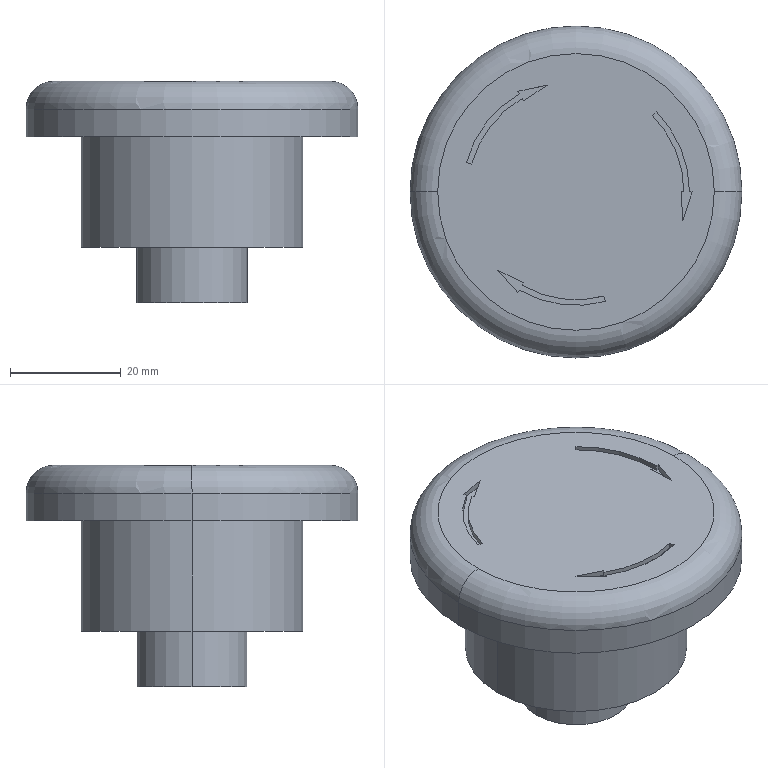Part | SolidWorks | features ICE 3, CirPattern 1, Extrusion 1, Fillet 1, Scale 1 | 1 solid | 36 faces | box 60 x 60 x 40 mm | volume 55512 mm3 | plane 22 | cylinder 12 | torus 2 | commonest cylinder face diameters 39 x3 41 x3 20 x2 40 x2 60 x2
STEP:
#1=CARTESIAN_POINT('',(-3.,0.,27.294));
#2=VERTEX_POINT('',#1);
#3=CARTESIAN_POINT('',(3.,0.,27.294));
#4=VERTEX_POINT('',#3);
#5=CARTESIAN_POINT('',(0.,0.,27.294));
#6=DIRECTION('',(0.,0.,-1.));
#7=DIRECTION('',(1.,0.,0.));
#8=AXIS2_PLACEMENT_3D('',#5,#6,#7);
#9=CIRCLE('',#8,3.);
#10=EDGE_CURVE('',#2,#4,#9,.T.);
#11=ORIENTED_EDGE('',*,*,#10,.F.);
#12=CARTESIAN_POINT('',(-2.5,0.,27.794));
#13=VERTEX_POINT('',#12);
#14=CARTESIAN_POINT('',(-2.5,0.,27.294));
#15=DIRECTION('',(0.,1.,0.));
#16=DIRECTION('',(-1.,0.,0.));
#17=AXIS2_PLACEMENT_3D('',#14,#15,#16);
#18=CIRCLE('',#17,0.5);
#19=EDGE_CURVE('',#2,#13,#18,.T.);
#20=ORIENTED_EDGE('',*,*,#19,.T.);
#21=CARTESIAN_POINT('',(2.5,0.,27.794));
#22=VERTEX_POINT('',#21);
#23=CARTESIAN_POINT('',(0.,0.,27.794));
#24=DIRECTION('',(0.,0.,1.));
#25=DIRECTION('',(1.,0.,0.));
#26=AXIS2_PLACEMENT_3D('',#23,#24,#25);
#27=CIRCLE('',#26,2.5);
#28=EDGE_CURVE('',#22,#13,#27,.T.);
#29=ORIENTED_EDGE('',*,*,#28,.F.);
#30=CARTESIAN_POINT('',(2.5,0.,27.294));
#31=DIRECTION('',(0.,-1.,0.));
#32=DIRECTION('',(0.,0.,-1.));
#33=AXIS2_PLACEMENT_3D('',#30,#31,#32);
#34=CIRCLE('',#33,0.5);
#35=EDGE_CURVE('',#4,#22,#34,.T.);
#36=ORIENTED_EDGE('',*,*,#35,.F.);
#37=EDGE_LOOP('',(#11,#20,#29,#36));
#38=FACE_OUTER_BOUND('',#37,.T.);
#39=CARTESIAN_POINT('',(0.,0.,27.294));
#40=DIRECTION('',(0.,0.,1.));
#41=DIRECTION('',(1.,0.,0.));
#42=AXIS2_PLACEMENT_3D('',#39,#40,#41);
#43=TOROIDAL_SURFACE('',#42,2.5,0.5);
#44=ADVANCED_FACE('',(#38),#43,.T.);
#45=ORIENTED_EDGE('',*,*,#10,.T.);
#46=CARTESIAN_POINT('',(3.,0.,26.794));
#47=VERTEX_POINT('',#46);
#48=CARTESIAN_POINT('',(3.,0.,27.794));
#49=DIRECTION('',(0.,0.,-1.));
#50=VECTOR('',#49,100.);
#51=LINE('',#48,#50);
#52=EDGE_CURVE('',#4,#47,#51,.T.);
#53=ORIENTED_EDGE('',*,*,#52,.T.);
#54=CARTESIAN_POINT('',(-3.,0.,26.794));
#55=VERTEX_POINT('',#54);
#56=CARTESIAN_POINT('',(0.,0.,26.794));
#57=DIRECTION('',(0.,0.,1.));
#58=DIRECTION('',(1.,0.,0.));
#59=AXIS2_PLACEMENT_3D('',#56,#57,#58);
#60=CIRCLE('',#59,3.);
#61=EDGE_CURVE('',#47,#55,#60,.T.);
#62=ORIENTED_EDGE('',*,*,#61,.T.);
#63=CARTESIAN_POINT('',(-3.,0.,27.794));
#64=DIRECTION('',(0.,0.,-1.));
#65=VECTOR('',#64,100.);
#66=LINE('',#63,#65);
#67=EDGE_CURVE('',#2,#55,#66,.T.);
#68=ORIENTED_EDGE('',*,*,#67,.F.);
#69=EDGE_LOOP('',(#45,#53,#62,#68));
#70=FACE_OUTER_BOUND('',#69,.T.);
#71=CARTESIAN_POINT('',(0.,0.,27.794));
#72=DIRECTION('',(0.,0.,-1.));
#73=DIRECTION('',(-1.,0.,0.));
#74=AXIS2_PLACEMENT_3D('',#71,#72,#73);
#75=CYLINDRICAL_SURFACE('',#74,3.);
#76=ADVANCED_FACE('',(#70),#75,.T.);
#77=CARTESIAN_POINT('',(2.,0.,26.794));
#78=VERTEX_POINT('',#77);
#79=CARTESIAN_POINT('',(-2.,0.,26.794));
#80=VERTEX_POINT('',#79);
#81=CARTESIAN_POINT('',(0.,0.,26.794));
#82=DIRECTION('',(0.,0.,1.));
#83=DIRECTION('',(1.,0.,0.));
#84=AXIS2_PLACEMENT_3D('',#81,#82,#83);
#85=CIRCLE('',#84,2.);
#86=EDGE_CURVE('',#78,#80,#85,.T.);
#87=ORIENTED_EDGE('',*,*,#86,.F.);
#88=CARTESIAN_POINT('',(2.,0.,24.794));
#89=VERTEX_POINT('',#88);
#90=CARTESIAN_POINT('',(2.,0.,26.794));
#91=DIRECTION('',(0.,0.,-1.));
#92=VECTOR('',#91,100.);
#93=LINE('',#90,#92);
#94=EDGE_CURVE('',#78,#89,#93,.T.);
#95=ORIENTED_EDGE('',*,*,#94,.T.);
#96=CARTESIAN_POINT('',(-2.,0.,24.794));
#97=VERTEX_POINT('',#96);
#98=CARTESIAN_POINT('',(0.,0.,24.794));
#99=DIRECTION('',(0.,0.,1.));
#100=DIRECTION('',(1.,0.,0.));
#101=AXIS2_PLACEMENT_3D('',#98,#99,#100);
#102=CIRCLE('',#101,2.);
#103=EDGE_CURVE('',#89,#97,#102,.T.);
#104=ORIENTED_EDGE('',*,*,#103,.T.);
#105=CARTESIAN_POINT('',(-2.,0.,26.794));
#106=DIRECTION('',(0.,0.,-1.));
#107=VECTOR('',#106,100.);
#108=LINE('',#105,#107);
#109=EDGE_CURVE('',#80,#97,#108,.T.);
#110=ORIENTED_EDGE('',*,*,#109,.F.);
#111=EDGE_LOOP('',(#87,#95,#104,#110));
#112=FACE_OUTER_BOUND('',#111,.T.);
#113=CARTESIAN_POINT('',(0.,0.,26.794));
#114=DIRECTION('',(0.,0.,-1.));
#115=DIRECTION('',(-1.,0.,0.));
#116=AXIS2_PLACEMENT_3D('',#113,#114,#115);
#117=CYLINDRICAL_SURFACE('',#116,2.);
#118=ADVANCED_FACE('',(#112),#117,.T.);
#119=CARTESIAN_POINT('',(1.,0.,24.794));
#120=VERTEX_POINT('',#119);
#121=CARTESIAN_POINT('',(-1.,0.,24.794));
#122=VERTEX_POINT('',#121);
#123=CARTESIAN_POINT('',(0.,0.,24.794));
#124=DIRECTION('',(0.,0.,1.));
#125=DIRECTION('',(1.,0.,0.));
#126=AXIS2_PLACEMENT_3D('',#123,#124,#125);
#127=CIRCLE('',#126,1.);
#128=EDGE_CURVE('',#120,#122,#127,.T.);
#129=ORIENTED_EDGE('',*,*,#128,.F.);
#130=CARTESIAN_POINT('',(1.,0.,23.794));
#131=VERTEX_POINT('',#130);
#132=CARTESIAN_POINT('',(1.,0.,24.794));
#133=DIRECTION('',(0.,0.,-1.));
#134=VECTOR('',#133,100.);
#135=LINE('',#132,#134);
#136=EDGE_CURVE('',#120,#131,#135,.T.);
#137=ORIENTED_EDGE('',*,*,#136,.T.);
#138=CARTESIAN_POINT('',(-1.,0.,23.794));
#139=VERTEX_POINT('',#138);
#140=CARTESIAN_POINT('',(0.,0.,23.794));
#141=DIRECTION('',(0.,0.,1.));
#142=DIRECTION('',(1.,0.,0.));
#143=AXIS2_PLACEMENT_3D('',#140,#141,#142);
#144=CIRCLE('',#143,1.);
#145=EDGE_CURVE('',#131,#139,#144,.T.);
#146=ORIENTED_EDGE('',*,*,#145,.T.);
#147=CARTESIAN_POINT('',(-1.,0.,24.794));
#148=DIRECTION('',(0.,0.,-1.));
#149=VECTOR('',#148,100.);
#150=LINE('',#147,#149);
#151=EDGE_CURVE('',#122,#139,#150,.T.);
#152=ORIENTED_EDGE('',*,*,#151,.F.);
#153=EDGE_LOOP('',(#129,#137,#146,#152));
#154=FACE_OUTER_BOUND('',#153,.T.);
#155=CARTESIAN_POINT('',(0.,0.,24.794));
#156=DIRECTION('',(0.,0.,-1.));
#157=DIRECTION('',(-1.,0.,0.));
#158=AXIS2_PLACEMENT_3D('',#155,#156,#157);
#159=CYLINDRICAL_SURFACE('',#158,1.);
#160=ADVANCED_FACE('',(#154),#159,.T.);
#161=ORIENTED_EDGE('',*,*,#136,.F.);
#162=CARTESIAN_POINT('',(0.,0.,24.794));
#163=DIRECTION('',(0.,0.,1.));
#164=DIRECTION('',(1.,0.,0.));
#165=AXIS2_PLACEMENT_3D('',#162,#163,#164);
#166=CIRCLE('',#165,1.);
#167=EDGE_CURVE('',#122,#120,#166,.T.);
#168=ORIENTED_EDGE('',*,*,#167,.F.);
#169=ORIENTED_EDGE('',*,*,#151,.T.);
#170=CARTESIAN_POINT('',(0.,0.,23.794));
#171=DIRECTION('',(0.,0.,1.));
#172=DIRECTION('',(1.,0.,0.));
#173=AXIS2_PLACEMENT_3D('',#170,#171,#172);
#174=CIRCLE('',#173,1.);
#175=EDGE_CURVE('',#139,#131,#174,.T.);
#176=ORIENTED_EDGE('',*,*,#175,.T.);
#177=EDGE_LOOP('',(#161,#168,#169,#176));
#178=FACE_OUTER_BOUND('',#177,.T.);
#179=CARTESIAN_POINT('',(0.,0.,24.794));
#180=DIRECTION('',(0.,0.,-1.));
#181=DIRECTION('',(-1.,0.,0.));
#182=AXIS2_PLACEMENT_3D('',#179,#180,#181);
#183=CYLINDRICAL_SURFACE('',#182,1.);
#184=ADVANCED_FACE('',(#178),#183,.T.);
#185=ORIENTED_EDGE('',*,*,#175,.F.);
#186=ORIENTED_EDGE('',*,*,#145,.F.);
#187=EDGE_LOOP('',(#185,#186));
#188=FACE_OUTER_BOUND('',#187,.T.);
#189=CARTESIAN_POINT('',(0.,0.,23.794));
#190=DIRECTION('',(0.,0.,1.));
#191=DIRECTION('',(1.,0.,0.));
#192=AXIS2_PLACEMENT_3D('',#189,#190,#191);
#193=PLANE('',#192);
#194=ADVANCED_FACE('',(#188),#193,.F.);
#195=ORIENTED_EDGE('',*,*,#94,.F.);
#196=CARTESIAN_POINT('',(0.,0.,26.794));
#197=DIRECTION('',(0.,0.,1.));
#198=DIRECTION('',(1.,0.,0.));
#199=AXIS2_PLACEMENT_3D('',#196,#197,#198);
#200=CIRCLE('',#199,2.);
#201=EDGE_CURVE('',#80,#78,#200,.T.);
#202=ORIENTED_EDGE('',*,*,#201,.F.);
#203=ORIENTED_EDGE('',*,*,#109,.T.);
#204=CARTESIAN_POINT('',(0.,0.,24.794));
#205=DIRECTION('',(0.,0.,1.));
#206=DIRECTION('',(1.,0.,0.));
#207=AXIS2_PLACEMENT_3D('',#204,#205,#206);
#208=CIRCLE('',#207,2.);
#209=EDGE_CURVE('',#97,#89,#208,.T.);
#210=ORIENTED_EDGE('',*,*,#209,.T.);
#211=EDGE_LOOP('',(#195,#202,#203,#210));
#212=FACE_OUTER_BOUND('',#211,.T.);
#213=CARTESIAN_POINT('',(0.,0.,26.794));
#214=DIRECTION('',(0.,0.,-1.));
#215=DIRECTION('',(-1.,0.,0.));
#216=AXIS2_PLACEMENT_3D('',#213,#214,#215);
#217=CYLINDRICAL_SURFACE('',#216,2.);
#218=ADVANCED_FACE('',(#212),#217,.T.);
#219=ORIENTED_EDGE('',*,*,#167,.T.);
#220=ORIENTED_EDGE('',*,*,#128,.T.);
#221=EDGE_LOOP('',(#219,#220));
#222=FACE_BOUND('',#221,.T.);
#223=ORIENTED_EDGE('',*,*,#209,.F.);
#224=ORIENTED_EDGE('',*,*,#103,.F.);
#225=EDGE_LOOP('',(#223,#224));
#226=FACE_OUTER_BOUND('',#225,.T.);
#227=CARTESIAN_POINT('',(0.,0.,24.794));
#228=DIRECTION('',(0.,0.,1.));
#229=DIRECTION('',(1.,0.,0.));
#230=AXIS2_PLACEMENT_3D('',#227,#228,#229);
#231=PLANE('',#230);
#232=ADVANCED_FACE('',(#222,#226),#231,.F.);
#233=ORIENTED_EDGE('',*,*,#52,.F.);
#234=CARTESIAN_POINT('',(0.,0.,27.294));
#235=DIRECTION('',(0.,0.,-1.));
#236=DIRECTION('',(1.,0.,0.));
#237=AXIS2_PLACEMENT_3D('',#234,#235,#236);
#238=CIRCLE('',#237,3.);
#239=EDGE_CURVE('',#4,#2,#238,.T.);
#240=ORIENTED_EDGE('',*,*,#239,.T.);
#241=ORIENTED_EDGE('',*,*,#67,.T.);
#242=CARTESIAN_POINT('',(0.,0.,26.794));
#243=DIRECTION('',(0.,0.,1.));
#244=DIRECTION('',(1.,0.,0.));
#245=AXIS2_PLACEMENT_3D('',#242,#243,#244);
#246=CIRCLE('',#245,3.);
#247=EDGE_CURVE('',#55,#47,#246,.T.);
#248=ORIENTED_EDGE('',*,*,#247,.T.);
#249=EDGE_LOOP('',(#233,#240,#241,#248));
#250=FACE_OUTER_BOUND('',#249,.T.);
#251=CARTESIAN_POINT('',(0.,0.,27.794));
#252=DIRECTION('',(0.,0.,-1.));
#253=DIRECTION('',(-1.,0.,0.));
#254=AXIS2_PLACEMENT_3D('',#251,#252,#253);
#255=CYLINDRICAL_SURFACE('',#254,3.);
#256=ADVANCED_FACE('',(#250),#255,.T.);
#257=ORIENTED_EDGE('',*,*,#28,.T.);
#258=CARTESIAN_POINT('',(0.,0.,27.794));
#259=DIRECTION('',(0.,0.,1.));
#260=DIRECTION('',(1.,0.,0.));
#261=AXIS2_PLACEMENT_3D('',#258,#259,#260);
#262=CIRCLE('',#261,2.5);
#263=EDGE_CURVE('',#13,#22,#262,.T.);
#264=ORIENTED_EDGE('',*,*,#263,.T.);
#265=EDGE_LOOP('',(#257,#264));
#266=FACE_OUTER_BOUND('',#265,.T.);
#267=CARTESIAN_POINT('',(0.5047,-1.884,27.794));
#268=VERTEX_POINT('',#267);
#269=CARTESIAN_POINT('',(-0.975,-1.689,27.794));
#270=VERTEX_POINT('',#269);
#271=CARTESIAN_POINT('',(0.,0.,27.794));
#272=DIRECTION('',(0.,0.,-1.));
#273=DIRECTION('',(-0.5,0.866,0.));
#274=AXIS2_PLACEMENT_3D('',#271,#272,#273);
#275=CIRCLE('',#274,1.95);
#276=EDGE_CURVE('',#268,#270,#275,.T.);
#277=ORIENTED_EDGE('',*,*,#276,.F.);
#278=CARTESIAN_POINT('',(0.5306,-1.98,27.794));
#279=VERTEX_POINT('',#278);
#280=CARTESIAN_POINT('',(0.5047,-1.884,27.794));
#281=DIRECTION('',(-0.2588,0.9659,0.));
#282=VECTOR('',#281,100.);
#283=LINE('',#280,#282);
#284=EDGE_CURVE('',#279,#268,#283,.T.);
#285=ORIENTED_EDGE('',*,*,#284,.F.);
#286=CARTESIAN_POINT('',(-1.025,-1.775,27.794));
#287=VERTEX_POINT('',#286);
#288=CARTESIAN_POINT('',(0.,0.,27.794));
#289=DIRECTION('',(0.,0.,1.));
#290=DIRECTION('',(-0.5,0.866,0.));
#291=AXIS2_PLACEMENT_3D('',#288,#289,#290);
#292=CIRCLE('',#291,2.05);
#293=EDGE_CURVE('',#287,#279,#292,.T.);
#294=ORIENTED_EDGE('',*,*,#293,.F.);
#295=CARTESIAN_POINT('',(-1.05,-1.819,27.794));
#296=VERTEX_POINT('',#295);
#297=CARTESIAN_POINT('',(-1.05,-1.819,27.794));
#298=DIRECTION('',(0.5,0.866,0.));
#299=VECTOR('',#298,100.);
#300=LINE('',#297,#299);
#301=EDGE_CURVE('',#296,#287,#300,.T.);
#302=ORIENTED_EDGE('',*,*,#301,.F.);
#303=CARTESIAN_POINT('',(-1.414,-1.414,27.794));
#304=VERTEX_POINT('',#303);
#305=CARTESIAN_POINT('',(-1.05,-1.819,27.794));
#306=DIRECTION('',(0.6692,-0.7431,0.));
#307=VECTOR('',#306,100.);
#308=LINE('',#305,#307);
#309=EDGE_CURVE('',#304,#296,#308,.T.);
#310=ORIENTED_EDGE('',*,*,#309,.F.);
#311=CARTESIAN_POINT('',(-0.95,-1.645,27.794));
#312=VERTEX_POINT('',#311);
#313=CARTESIAN_POINT('',(-0.95,-1.645,27.794));
#314=DIRECTION('',(-0.8951,0.4459,0.));
#315=VECTOR('',#314,100.);
#316=LINE('',#313,#315);
#317=EDGE_CURVE('',#312,#304,#316,.T.);
#318=ORIENTED_EDGE('',*,*,#317,.F.);
#319=CARTESIAN_POINT('',(-0.975,-1.689,27.794));
#320=DIRECTION('',(0.5,0.866,0.));
#321=VECTOR('',#320,100.);
#322=LINE('',#319,#321);
#323=EDGE_CURVE('',#270,#312,#322,.T.);
#324=ORIENTED_EDGE('',*,*,#323,.F.);
#325=EDGE_LOOP('',(#277,#285,#294,#302,#310,#318,#324));
#326=FACE_BOUND('',#325,.T.);
#327=CARTESIAN_POINT('',(1.379,1.379,27.794));
#328=VERTEX_POINT('',#327);
#329=CARTESIAN_POINT('',(1.95,0.,27.794));
#330=VERTEX_POINT('',#329);
#331=CARTESIAN_POINT('',(0.,0.,27.794));
#332=DIRECTION('',(0.,0.,-1.));
#333=DIRECTION('',(-0.5,-0.866,0.));
#334=AXIS2_PLACEMENT_3D('',#331,#332,#333);
#335=CIRCLE('',#334,1.95);
#336=EDGE_CURVE('',#328,#330,#335,.T.);
#337=ORIENTED_EDGE('',*,*,#336,.F.);
#338=CARTESIAN_POINT('',(1.45,1.45,27.794));
#339=VERTEX_POINT('',#338);
#340=CARTESIAN_POINT('',(1.379,1.379,27.794));
#341=DIRECTION('',(-0.7071,-0.7071,0.));
#342=VECTOR('',#341,100.);
#343=LINE('',#340,#342);
#344=EDGE_CURVE('',#339,#328,#343,.T.);
#345=ORIENTED_EDGE('',*,*,#344,.F.);
#346=CARTESIAN_POINT('',(2.05,0.,27.794));
#347=VERTEX_POINT('',#346);
#348=CARTESIAN_POINT('',(0.,0.,27.794));
#349=DIRECTION('',(0.,0.,1.));
#350=DIRECTION('',(-0.5,-0.866,0.));
#351=AXIS2_PLACEMENT_3D('',#348,#349,#350);
#352=CIRCLE('',#351,2.05);
#353=EDGE_CURVE('',#347,#339,#352,.T.);
#354=ORIENTED_EDGE('',*,*,#353,.F.);
#355=CARTESIAN_POINT('',(2.1,0.,27.794));
#356=VERTEX_POINT('',#355);
#357=CARTESIAN_POINT('',(2.1,0.,27.794));
#358=DIRECTION('',(-1.,0.,0.));
#359=VECTOR('',#358,100.);
#360=LINE('',#357,#359);
#361=EDGE_CURVE('',#356,#347,#360,.T.);
#362=ORIENTED_EDGE('',*,*,#361,.F.);
#363=CARTESIAN_POINT('',(1.932,-0.5176,27.794));
#364=VERTEX_POINT('',#363);
#365=CARTESIAN_POINT('',(2.1,0.,27.794));
#366=DIRECTION('',(0.3089,0.9511,0.));
#367=VECTOR('',#366,100.);
#368=LINE('',#365,#367);
#369=EDGE_CURVE('',#364,#356,#368,.T.);
#370=ORIENTED_EDGE('',*,*,#369,.F.);
#371=CARTESIAN_POINT('',(1.9,0.,27.794));
#372=VERTEX_POINT('',#371);
#373=CARTESIAN_POINT('',(1.9,0.,27.794));
#374=DIRECTION('',(0.06142,-0.9981,0.));
#375=VECTOR('',#374,100.);
#376=LINE('',#373,#375);
#377=EDGE_CURVE('',#372,#364,#376,.T.);
#378=ORIENTED_EDGE('',*,*,#377,.F.);
#379=CARTESIAN_POINT('',(1.95,0.,27.794));
#380=DIRECTION('',(-1.,0.,0.));
#381=VECTOR('',#380,100.);
#382=LINE('',#379,#381);
#383=EDGE_CURVE('',#330,#372,#382,.T.);
#384=ORIENTED_EDGE('',*,*,#383,.F.);
#385=EDGE_LOOP('',(#337,#345,#354,#362,#370,#378,#384));
#386=FACE_BOUND('',#385,.T.);
#387=CARTESIAN_POINT('',(-1.884,0.5047,27.794));
#388=VERTEX_POINT('',#387);
#389=CARTESIAN_POINT('',(-0.975,1.689,27.794));
#390=VERTEX_POINT('',#389);
#391=CARTESIAN_POINT('',(0.,0.,27.794));
#392=DIRECTION('',(0.,0.,-1.));
#393=DIRECTION('',(1.,0.,0.));
#394=AXIS2_PLACEMENT_3D('',#391,#392,#393);
#395=CIRCLE('',#394,1.95);
#396=EDGE_CURVE('',#388,#390,#395,.T.);
#397=ORIENTED_EDGE('',*,*,#396,.F.);
#398=CARTESIAN_POINT('',(-1.98,0.5306,27.794));
#399=VERTEX_POINT('',#398);
#400=CARTESIAN_POINT('',(-1.884,0.5047,27.794));
#401=DIRECTION('',(0.9659,-0.2588,0.));
#402=VECTOR('',#401,100.);
#403=LINE('',#400,#402);
#404=EDGE_CURVE('',#399,#388,#403,.T.);
#405=ORIENTED_EDGE('',*,*,#404,.F.);
#406=CARTESIAN_POINT('',(-1.025,1.775,27.794));
#407=VERTEX_POINT('',#406);
#408=CARTESIAN_POINT('',(0.,0.,27.794));
#409=DIRECTION('',(0.,0.,1.));
#410=DIRECTION('',(1.,0.,0.));
#411=AXIS2_PLACEMENT_3D('',#408,#409,#410);
#412=CIRCLE('',#411,2.05);
#413=EDGE_CURVE('',#407,#399,#412,.T.);
#414=ORIENTED_EDGE('',*,*,#413,.F.);
#415=CARTESIAN_POINT('',(-1.05,1.819,27.794));
#416=VERTEX_POINT('',#415);
#417=CARTESIAN_POINT('',(-1.05,1.819,27.794));
#418=DIRECTION('',(0.5,-0.866,0.));
#419=VECTOR('',#418,100.);
#420=LINE('',#417,#419);
#421=EDGE_CURVE('',#416,#407,#420,.T.);
#422=ORIENTED_EDGE('',*,*,#421,.F.);
#423=CARTESIAN_POINT('',(-0.5176,1.932,27.794));
#424=VERTEX_POINT('',#423);
#425=CARTESIAN_POINT('',(-1.05,1.819,27.794));
#426=DIRECTION('',(-0.9781,-0.208,0.));
#427=VECTOR('',#426,100.);
#428=LINE('',#425,#427);
#429=EDGE_CURVE('',#424,#416,#428,.T.);
#430=ORIENTED_EDGE('',*,*,#429,.F.);
#431=CARTESIAN_POINT('',(-0.95,1.645,27.794));
#432=VERTEX_POINT('',#431);
#433=CARTESIAN_POINT('',(-0.95,1.645,27.794));
#434=DIRECTION('',(0.8337,0.5522,0.));
#435=VECTOR('',#434,100.);
#436=LINE('',#433,#435);
#437=EDGE_CURVE('',#432,#424,#436,.T.);
#438=ORIENTED_EDGE('',*,*,#437,.F.);
#439=CARTESIAN_POINT('',(-0.975,1.689,27.794));
#440=DIRECTION('',(0.5,-0.866,0.));
#441=VECTOR('',#440,100.);
#442=LINE('',#439,#441);
#443=EDGE_CURVE('',#390,#432,#442,.T.);
#444=ORIENTED_EDGE('',*,*,#443,.F.);
#445=EDGE_LOOP('',(#397,#405,#414,#422,#430,#438,#444));
#446=FACE_BOUND('',#445,.T.);
#447=CARTESIAN_POINT('',(0.,0.,27.794));
#448=DIRECTION('',(0.,0.,1.));
#449=DIRECTION('',(1.,0.,0.));
#450=AXIS2_PLACEMENT_3D('',#447,#448,#449);
#451=PLANE('',#450);
#452=ADVANCED_FACE('',(#266,#326,#386,#446),#451,.T.);
#453=ORIENTED_EDGE('',*,*,#201,.T.);
#454=ORIENTED_EDGE('',*,*,#86,.T.);
#455=EDGE_LOOP('',(#453,#454));
#456=FACE_BOUND('',#455,.T.);
#457=ORIENTED_EDGE('',*,*,#247,.F.);
#458=ORIENTED_EDGE('',*,*,#61,.F.);
#459=EDGE_LOOP('',(#457,#458));
#460=FACE_OUTER_BOUND('',#459,.T.);
#461=CARTESIAN_POINT('',(0.,0.,26.794));
#462=DIRECTION('',(0.,0.,1.));
#463=DIRECTION('',(1.,0.,0.));
#464=AXIS2_PLACEMENT_3D('',#461,#462,#463);
#465=PLANE('',#464);
#466=ADVANCED_FACE('',(#456,#460),#465,.F.);
#467=ORIENTED_EDGE('',*,*,#396,.T.);
#468=CARTESIAN_POINT('',(-0.975,1.689,27.694));
#469=VERTEX_POINT('',#468);
#470=CARTESIAN_POINT('',(-0.975,1.689,27.694));
#471=DIRECTION('',(0.,0.,1.));
#472=VECTOR('',#471,100.);
#473=LINE('',#470,#472);
#474=EDGE_CURVE('',#469,#390,#473,.T.);
#475=ORIENTED_EDGE('',*,*,#474,.F.);
#476=CARTESIAN_POINT('',(-1.884,0.5047,27.694));
#477=VERTEX_POINT('',#476);
#478=CARTESIAN_POINT('',(0.,0.,27.694));
#479=DIRECTION('',(0.,0.,-1.));
#480=DIRECTION('',(1.,0.,0.));
#481=AXIS2_PLACEMENT_3D('',#478,#479,#480);
#482=CIRCLE('',#481,1.95);
#483=EDGE_CURVE('',#477,#469,#482,.T.);
#484=ORIENTED_EDGE('',*,*,#483,.F.);
#485=CARTESIAN_POINT('',(-1.884,0.5047,27.694));
#486=DIRECTION('',(0.,0.,1.));
#487=VECTOR('',#486,100.);
#488=LINE('',#485,#487);
#489=EDGE_CURVE('',#477,#388,#488,.T.);
#490=ORIENTED_EDGE('',*,*,#489,.T.);
#491=EDGE_LOOP('',(#467,#475,#484,#490));
#492=FACE_OUTER_BOUND('',#491,.T.);
#493=CARTESIAN_POINT('',(0.,0.,27.694));
#494=DIRECTION('',(0.,0.,1.));
#495=DIRECTION('',(1.,0.,0.));
#496=AXIS2_PLACEMENT_3D('',#493,#494,#495);
#497=CYLINDRICAL_SURFACE('',#496,1.95);
#498=ADVANCED_FACE('',(#492),#497,.T.);
#499=ORIENTED_EDGE('',*,*,#404,.T.);
#500=ORIENTED_EDGE('',*,*,#489,.F.);
#501=CARTESIAN_POINT('',(-1.98,0.5306,27.694));
#502=VERTEX_POINT('',#501);
#503=CARTESIAN_POINT('',(-1.884,0.5047,27.694));
#504=DIRECTION('',(0.9659,-0.2588,0.));
#505=VECTOR('',#504,100.);
#506=LINE('',#503,#505);
#507=EDGE_CURVE('',#502,#477,#506,.T.);
#508=ORIENTED_EDGE('',*,*,#507,.F.);
#509=CARTESIAN_POINT('',(-1.98,0.5306,27.694));
#510=DIRECTION('',(0.,0.,1.));
#511=VECTOR('',#510,100.);
#512=LINE('',#509,#511);
#513=EDGE_CURVE('',#502,#399,#512,.T.);
#514=ORIENTED_EDGE('',*,*,#513,.T.);
#515=EDGE_LOOP('',(#499,#500,#508,#514));
#516=FACE_OUTER_BOUND('',#515,.T.);
#517=CARTESIAN_POINT('',(-1.884,0.5047,27.694));
#518=DIRECTION('',(-0.2588,-0.9659,0.));
#519=DIRECTION('',(0.9659,-0.2588,0.));
#520=AXIS2_PLACEMENT_3D('',#517,#518,#519);
#521=PLANE('',#520);
#522=ADVANCED_FACE('',(#516),#521,.F.);
#523=ORIENTED_EDGE('',*,*,#413,.T.);
#524=ORIENTED_EDGE('',*,*,#513,.F.);
#525=CARTESIAN_POINT('',(-1.025,1.775,27.694));
#526=VERTEX_POINT('',#525);
#527=CARTESIAN_POINT('',(0.,0.,27.694));
#528=DIRECTION('',(0.,0.,1.));
#529=DIRECTION('',(1.,0.,0.));
#530=AXIS2_PLACEMENT_3D('',#527,#528,#529);
#531=CIRCLE('',#530,2.05);
#532=EDGE_CURVE('',#526,#502,#531,.T.);
#533=ORIENTED_EDGE('',*,*,#532,.F.);
#534=CARTESIAN_POINT('',(-1.025,1.775,27.694));
#535=DIRECTION('',(0.,0.,1.));
#536=VECTOR('',#535,100.);
#537=LINE('',#534,#536);
#538=EDGE_CURVE('',#526,#407,#537,.T.);
#539=ORIENTED_EDGE('',*,*,#538,.T.);
#540=EDGE_LOOP('',(#523,#524,#533,#539));
#541=FACE_OUTER_BOUND('',#540,.T.);
#542=CARTESIAN_POINT('',(0.,0.,27.694));
#543=DIRECTION('',(0.,0.,1.));
#544=DIRECTION('',(1.,0.,0.));
#545=AXIS2_PLACEMENT_3D('',#542,#543,#544);
#546=CYLINDRICAL_SURFACE('',#545,2.05);
#547=ADVANCED_FACE('',(#541),#546,.F.);
#548=ORIENTED_EDGE('',*,*,#421,.T.);
#549=ORIENTED_EDGE('',*,*,#538,.F.);
#550=CARTESIAN_POINT('',(-1.05,1.819,27.694));
#551=VERTEX_POINT('',#550);
#552=CARTESIAN_POINT('',(-1.05,1.819,27.694));
#553=DIRECTION('',(0.5,-0.866,0.));
#554=VECTOR('',#553,100.);
#555=LINE('',#552,#554);
#556=EDGE_CURVE('',#551,#526,#555,.T.);
#557=ORIENTED_EDGE('',*,*,#556,.F.);
#558=CARTESIAN_POINT('',(-1.05,1.819,27.694));
#559=DIRECTION('',(0.,0.,1.));
#560=VECTOR('',#559,100.);
#561=LINE('',#558,#560);
#562=EDGE_CURVE('',#551,#416,#561,.T.);
#563=ORIENTED_EDGE('',*,*,#562,.T.);
#564=EDGE_LOOP('',(#548,#549,#557,#563));
#565=FACE_OUTER_BOUND('',#564,.T.);
#566=CARTESIAN_POINT('',(-1.05,1.819,27.694));
#567=DIRECTION('',(-0.866,-0.5,0.));
#568=DIRECTION('',(0.5,-0.866,0.));
#569=AXIS2_PLACEMENT_3D('',#566,#567,#568);
#570=PLANE('',#569);
#571=ADVANCED_FACE('',(#565),#570,.F.);
#572=ORIENTED_EDGE('',*,*,#429,.T.);
#573=ORIENTED_EDGE('',*,*,#562,.F.);
#574=CARTESIAN_POINT('',(-0.5176,1.932,27.694));
#575=VERTEX_POINT('',#574);
#576=CARTESIAN_POINT('',(-1.05,1.819,27.694));
#577=DIRECTION('',(-0.9781,-0.208,0.));
#578=VECTOR('',#577,100.);
#579=LINE('',#576,#578);
#580=EDGE_CURVE('',#575,#551,#579,.T.);
#581=ORIENTED_EDGE('',*,*,#580,.F.);
#582=CARTESIAN_POINT('',(-0.5176,1.932,27.694));
#583=DIRECTION('',(0.,0.,1.));
#584=VECTOR('',#583,100.);
#585=LINE('',#582,#584);
#586=EDGE_CURVE('',#575,#424,#585,.T.);
#587=ORIENTED_EDGE('',*,*,#586,.T.);
#588=EDGE_LOOP('',(#572,#573,#581,#587));
#589=FACE_OUTER_BOUND('',#588,.T.);
#590=CARTESIAN_POINT('',(-1.05,1.819,27.694));
#591=DIRECTION('',(-0.208,0.9781,0.));
#592=DIRECTION('',(-0.9781,-0.208,0.));
#593=AXIS2_PLACEMENT_3D('',#590,#591,#592);
#594=PLANE('',#593);
#595=ADVANCED_FACE('',(#589),#594,.F.);
#596=ORIENTED_EDGE('',*,*,#437,.T.);
#597=ORIENTED_EDGE('',*,*,#586,.F.);
#598=CARTESIAN_POINT('',(-0.95,1.645,27.694));
#599=VERTEX_POINT('',#598);
#600=CARTESIAN_POINT('',(-0.95,1.645,27.694));
#601=DIRECTION('',(0.8337,0.5522,0.));
#602=VECTOR('',#601,100.);
#603=LINE('',#600,#602);
#604=EDGE_CURVE('',#599,#575,#603,.T.);
#605=ORIENTED_EDGE('',*,*,#604,.F.);
#606=CARTESIAN_POINT('',(-0.95,1.645,27.694));
#607=DIRECTION('',(0.,0.,1.));
#608=VECTOR('',#607,100.);
#609=LINE('',#606,#608);
#610=EDGE_CURVE('',#599,#432,#609,.T.);
#611=ORIENTED_EDGE('',*,*,#610,.T.);
#612=EDGE_LOOP('',(#596,#597,#605,#611));
#613=FACE_OUTER_BOUND('',#612,.T.);
#614=CARTESIAN_POINT('',(-0.95,1.645,27.694));
#615=DIRECTION('',(0.5522,-0.8337,0.));
#616=DIRECTION('',(0.8337,0.5522,0.));
#617=AXIS2_PLACEMENT_3D('',#614,#615,#616);
#618=PLANE('',#617);
#619=ADVANCED_FACE('',(#613),#618,.F.);
#620=ORIENTED_EDGE('',*,*,#443,.T.);
#621=ORIENTED_EDGE('',*,*,#610,.F.);
#622=CARTESIAN_POINT('',(-0.975,1.689,27.694));
#623=DIRECTION('',(0.5,-0.866,0.));
#624=VECTOR('',#623,100.);
#625=LINE('',#622,#624);
#626=EDGE_CURVE('',#469,#599,#625,.T.);
#627=ORIENTED_EDGE('',*,*,#626,.F.);
#628=ORIENTED_EDGE('',*,*,#474,.T.);
#629=EDGE_LOOP('',(#620,#621,#627,#628));
#630=FACE_OUTER_BOUND('',#629,.T.);
#631=CARTESIAN_POINT('',(-0.975,1.689,27.694));
#632=DIRECTION('',(-0.866,-0.5,0.));
#633=DIRECTION('',(0.5,-0.866,0.));
#634=AXIS2_PLACEMENT_3D('',#631,#632,#633);
#635=PLANE('',#634);
#636=ADVANCED_FACE('',(#630),#635,.F.);
#637=ORIENTED_EDGE('',*,*,#483,.T.);
#638=ORIENTED_EDGE('',*,*,#626,.T.);
#639=ORIENTED_EDGE('',*,*,#604,.T.);
#640=ORIENTED_EDGE('',*,*,#580,.T.);
#641=ORIENTED_EDGE('',*,*,#556,.T.);
#642=ORIENTED_EDGE('',*,*,#532,.T.);
#643=ORIENTED_EDGE('',*,*,#507,.T.);
#644=EDGE_LOOP('',(#637,#638,#639,#640,#641,#642,#643));
#645=FACE_OUTER_BOUND('',#644,.T.);
#646=CARTESIAN_POINT('',(0.,0.,27.694));
#647=DIRECTION('',(0.,0.,1.));
#648=DIRECTION('',(1.,0.,0.));
#649=AXIS2_PLACEMENT_3D('',#646,#647,#648);
#650=PLANE('',#649);
#651=ADVANCED_FACE('',(#645),#650,.T.);
#652=ORIENTED_EDGE('',*,*,#336,.T.);
#653=CARTESIAN_POINT('',(1.95,0.,27.694));
#654=VERTEX_POINT('',#653);
#655=CARTESIAN_POINT('',(1.95,0.,27.694));
#656=DIRECTION('',(0.,0.,1.));
#657=VECTOR('',#656,100.);
#658=LINE('',#655,#657);
#659=EDGE_CURVE('',#654,#330,#658,.T.);
#660=ORIENTED_EDGE('',*,*,#659,.F.);
#661=CARTESIAN_POINT('',(1.379,1.379,27.694));
#662=VERTEX_POINT('',#661);
#663=CARTESIAN_POINT('',(0.,0.,27.694));
#664=DIRECTION('',(0.,0.,-1.));
#665=DIRECTION('',(-0.5,-0.866,0.));
#666=AXIS2_PLACEMENT_3D('',#663,#664,#665);
#667=CIRCLE('',#666,1.95);
#668=EDGE_CURVE('',#662,#654,#667,.T.);
#669=ORIENTED_EDGE('',*,*,#668,.F.);
#670=CARTESIAN_POINT('',(1.379,1.379,27.694));
#671=DIRECTION('',(0.,0.,1.));
#672=VECTOR('',#671,100.);
#673=LINE('',#670,#672);
#674=EDGE_CURVE('',#662,#328,#673,.T.);
#675=ORIENTED_EDGE('',*,*,#674,.T.);
#676=EDGE_LOOP('',(#652,#660,#669,#675));
#677=FACE_OUTER_BOUND('',#676,.T.);
#678=CARTESIAN_POINT('',(0.,0.,27.694));
#679=DIRECTION('',(0.,0.,1.));
#680=DIRECTION('',(1.,0.,0.));
#681=AXIS2_PLACEMENT_3D('',#678,#679,#680);
#682=CYLINDRICAL_SURFACE('',#681,1.95);
#683=ADVANCED_FACE('',(#677),#682,.T.);
#684=ORIENTED_EDGE('',*,*,#344,.T.);
#685=ORIENTED_EDGE('',*,*,#674,.F.);
#686=CARTESIAN_POINT('',(1.45,1.45,27.694));
#687=VERTEX_POINT('',#686);
#688=CARTESIAN_POINT('',(1.379,1.379,27.694));
#689=DIRECTION('',(-0.7071,-0.7071,0.));
#690=VECTOR('',#689,100.);
#691=LINE('',#688,#690);
#692=EDGE_CURVE('',#687,#662,#691,.T.);
#693=ORIENTED_EDGE('',*,*,#692,.F.);
#694=CARTESIAN_POINT('',(1.45,1.45,27.694));
#695=DIRECTION('',(0.,0.,1.));
#696=VECTOR('',#695,100.);
#697=LINE('',#694,#696);
#698=EDGE_CURVE('',#687,#339,#697,.T.);
#699=ORIENTED_EDGE('',*,*,#698,.T.);
#700=EDGE_LOOP('',(#684,#685,#693,#699));
#701=FACE_OUTER_BOUND('',#700,.T.);
#702=CARTESIAN_POINT('',(1.379,1.379,27.694));
#703=DIRECTION('',(-0.7071,0.7071,0.));
#704=DIRECTION('',(-0.7071,-0.7071,0.));
#705=AXIS2_PLACEMENT_3D('',#702,#703,#704);
#706=PLANE('',#705);
#707=ADVANCED_FACE('',(#701),#706,.F.);
#708=ORIENTED_EDGE('',*,*,#353,.T.);
#709=ORIENTED_EDGE('',*,*,#698,.F.);
#710=CARTESIAN_POINT('',(2.05,0.,27.694));
#711=VERTEX_POINT('',#710);
#712=CARTESIAN_POINT('',(0.,0.,27.694));
#713=DIRECTION('',(0.,0.,1.));
#714=DIRECTION('',(-0.5,-0.866,0.));
#715=AXIS2_PLACEMENT_3D('',#712,#713,#714);
#716=CIRCLE('',#715,2.05);
#717=EDGE_CURVE('',#711,#687,#716,.T.);
#718=ORIENTED_EDGE('',*,*,#717,.F.);
#719=CARTESIAN_POINT('',(2.05,0.,27.694));
#720=DIRECTION('',(0.,0.,1.));
#721=VECTOR('',#720,100.);
#722=LINE('',#719,#721);
#723=EDGE_CURVE('',#711,#347,#722,.T.);
#724=ORIENTED_EDGE('',*,*,#723,.T.);
#725=EDGE_LOOP('',(#708,#709,#718,#724));
#726=FACE_OUTER_BOUND('',#725,.T.);
#727=CARTESIAN_POINT('',(0.,0.,27.694));
#728=DIRECTION('',(0.,0.,1.));
#729=DIRECTION('',(1.,0.,0.));
#730=AXIS2_PLACEMENT_3D('',#727,#728,#729);
#731=CYLINDRICAL_SURFACE('',#730,2.05);
#732=ADVANCED_FACE('',(#726),#731,.F.);
#733=ORIENTED_EDGE('',*,*,#361,.T.);
#734=ORIENTED_EDGE('',*,*,#723,.F.);
#735=CARTESIAN_POINT('',(2.1,0.,27.694));
#736=VERTEX_POINT('',#735);
#737=CARTESIAN_POINT('',(2.1,0.,27.694));
#738=DIRECTION('',(-1.,0.,0.));
#739=VECTOR('',#738,100.);
#740=LINE('',#737,#739);
#741=EDGE_CURVE('',#736,#711,#740,.T.);
#742=ORIENTED_EDGE('',*,*,#741,.F.);
#743=CARTESIAN_POINT('',(2.1,0.,27.694));
#744=DIRECTION('',(0.,0.,1.));
#745=VECTOR('',#744,100.);
#746=LINE('',#743,#745);
#747=EDGE_CURVE('',#736,#356,#746,.T.);
#748=ORIENTED_EDGE('',*,*,#747,.T.);
#749=EDGE_LOOP('',(#733,#734,#742,#748));
#750=FACE_OUTER_BOUND('',#749,.T.);
#751=CARTESIAN_POINT('',(2.1,0.,27.694));
#752=DIRECTION('',(0.,1.,0.));
#753=DIRECTION('',(-1.,0.,0.));
#754=AXIS2_PLACEMENT_3D('',#751,#752,#753);
#755=PLANE('',#754);
#756=ADVANCED_FACE('',(#750),#755,.F.);
#757=ORIENTED_EDGE('',*,*,#369,.T.);
#758=ORIENTED_EDGE('',*,*,#747,.F.);
#759=CARTESIAN_POINT('',(1.932,-0.5176,27.694));
#760=VERTEX_POINT('',#759);
#761=CARTESIAN_POINT('',(2.1,0.,27.694));
#762=DIRECTION('',(0.3089,0.9511,0.));
#763=VECTOR('',#762,100.);
#764=LINE('',#761,#763);
#765=EDGE_CURVE('',#760,#736,#764,.T.);
#766=ORIENTED_EDGE('',*,*,#765,.F.);
#767=CARTESIAN_POINT('',(1.932,-0.5176,27.694));
#768=DIRECTION('',(0.,0.,1.));
#769=VECTOR('',#768,100.);
#770=LINE('',#767,#769);
#771=EDGE_CURVE('',#760,#364,#770,.T.);
#772=ORIENTED_EDGE('',*,*,#771,.T.);
#773=EDGE_LOOP('',(#757,#758,#766,#772));
#774=FACE_OUTER_BOUND('',#773,.T.);
#775=CARTESIAN_POINT('',(2.1,0.,27.694));
#776=DIRECTION('',(0.9511,-0.3089,0.));
#777=DIRECTION('',(0.3089,0.9511,0.));
#778=AXIS2_PLACEMENT_3D('',#775,#776,#777);
#779=PLANE('',#778);
#780=ADVANCED_FACE('',(#774),#779,.F.);
#781=ORIENTED_EDGE('',*,*,#377,.T.);
#782=ORIENTED_EDGE('',*,*,#771,.F.);
#783=CARTESIAN_POINT('',(1.9,0.,27.694));
#784=VERTEX_POINT('',#783);
#785=CARTESIAN_POINT('',(1.9,0.,27.694));
#786=DIRECTION('',(0.06142,-0.9981,0.));
#787=VECTOR('',#786,100.);
#788=LINE('',#785,#787);
#789=EDGE_CURVE('',#784,#760,#788,.T.);
#790=ORIENTED_EDGE('',*,*,#789,.F.);
#791=CARTESIAN_POINT('',(1.9,0.,27.694));
#792=DIRECTION('',(0.,0.,1.));
#793=VECTOR('',#792,100.);
#794=LINE('',#791,#793);
#795=EDGE_CURVE('',#784,#372,#794,.T.);
#796=ORIENTED_EDGE('',*,*,#795,.T.);
#797=EDGE_LOOP('',(#781,#782,#790,#796));
#798=FACE_OUTER_BOUND('',#797,.T.);
#799=CARTESIAN_POINT('',(1.9,0.,27.694));
#800=DIRECTION('',(-0.9981,-0.06142,0.));
#801=DIRECTION('',(0.06142,-0.9981,0.));
#802=AXIS2_PLACEMENT_3D('',#799,#800,#801);
#803=PLANE('',#802);
#804=ADVANCED_FACE('',(#798),#803,.F.);
#805=ORIENTED_EDGE('',*,*,#383,.T.);
#806=ORIENTED_EDGE('',*,*,#795,.F.);
#807=CARTESIAN_POINT('',(1.95,0.,27.694));
#808=DIRECTION('',(-1.,0.,0.));
#809=VECTOR('',#808,100.);
#810=LINE('',#807,#809);
#811=EDGE_CURVE('',#654,#784,#810,.T.);
#812=ORIENTED_EDGE('',*,*,#811,.F.);
#813=ORIENTED_EDGE('',*,*,#659,.T.);
#814=EDGE_LOOP('',(#805,#806,#812,#813));
#815=FACE_OUTER_BOUND('',#814,.T.);
#816=CARTESIAN_POINT('',(1.95,0.,27.694));
#817=DIRECTION('',(0.,1.,0.));
#818=DIRECTION('',(-1.,0.,0.));
#819=AXIS2_PLACEMENT_3D('',#816,#817,#818);
#820=PLANE('',#819);
#821=ADVANCED_FACE('',(#815),#820,.F.);
#822=ORIENTED_EDGE('',*,*,#668,.T.);
#823=ORIENTED_EDGE('',*,*,#811,.T.);
#824=ORIENTED_EDGE('',*,*,#789,.T.);
#825=ORIENTED_EDGE('',*,*,#765,.T.);
#826=ORIENTED_EDGE('',*,*,#741,.T.);
#827=ORIENTED_EDGE('',*,*,#717,.T.);
#828=ORIENTED_EDGE('',*,*,#692,.T.);
#829=EDGE_LOOP('',(#822,#823,#824,#825,#826,#827,#828));
#830=FACE_OUTER_BOUND('',#829,.T.);
#831=CARTESIAN_POINT('',(0.,0.,27.694));
#832=DIRECTION('',(0.,0.,1.));
#833=DIRECTION('',(-0.5,-0.866,0.));
#834=AXIS2_PLACEMENT_3D('',#831,#832,#833);
#835=PLANE('',#834);
#836=ADVANCED_FACE('',(#830),#835,.T.);
#837=ORIENTED_EDGE('',*,*,#276,.T.);
#838=CARTESIAN_POINT('',(-0.975,-1.689,27.694));
#839=VERTEX_POINT('',#838);
#840=CARTESIAN_POINT('',(-0.975,-1.689,27.694));
#841=DIRECTION('',(0.,0.,1.));
#842=VECTOR('',#841,100.);
#843=LINE('',#840,#842);
#844=EDGE_CURVE('',#839,#270,#843,.T.);
#845=ORIENTED_EDGE('',*,*,#844,.F.);
#846=CARTESIAN_POINT('',(0.5047,-1.884,27.694));
#847=VERTEX_POINT('',#846);
#848=CARTESIAN_POINT('',(0.,0.,27.694));
#849=DIRECTION('',(0.,0.,-1.));
#850=DIRECTION('',(-0.5,0.866,0.));
#851=AXIS2_PLACEMENT_3D('',#848,#849,#850);
#852=CIRCLE('',#851,1.95);
#853=EDGE_CURVE('',#847,#839,#852,.T.);
#854=ORIENTED_EDGE('',*,*,#853,.F.);
#855=CARTESIAN_POINT('',(0.5047,-1.884,27.694));
#856=DIRECTION('',(0.,0.,1.));
#857=VECTOR('',#856,100.);
#858=LINE('',#855,#857);
#859=EDGE_CURVE('',#847,#268,#858,.T.);
#860=ORIENTED_EDGE('',*,*,#859,.T.);
#861=EDGE_LOOP('',(#837,#845,#854,#860));
#862=FACE_OUTER_BOUND('',#861,.T.);
#863=CARTESIAN_POINT('',(0.,0.,27.694));
#864=DIRECTION('',(0.,0.,1.));
#865=DIRECTION('',(1.,0.,0.));
#866=AXIS2_PLACEMENT_3D('',#863,#864,#865);
#867=CYLINDRICAL_SURFACE('',#866,1.95);
#868=ADVANCED_FACE('',(#862),#867,.T.);
#869=ORIENTED_EDGE('',*,*,#284,.T.);
#870=ORIENTED_EDGE('',*,*,#859,.F.);
#871=CARTESIAN_POINT('',(0.5306,-1.98,27.694));
#872=VERTEX_POINT('',#871);
#873=CARTESIAN_POINT('',(0.5047,-1.884,27.694));
#874=DIRECTION('',(-0.2588,0.9659,0.));
#875=VECTOR('',#874,100.);
#876=LINE('',#873,#875);
#877=EDGE_CURVE('',#872,#847,#876,.T.);
#878=ORIENTED_EDGE('',*,*,#877,.F.);
#879=CARTESIAN_POINT('',(0.5306,-1.98,27.694));
#880=DIRECTION('',(0.,0.,1.));
#881=VECTOR('',#880,100.);
#882=LINE('',#879,#881);
#883=EDGE_CURVE('',#872,#279,#882,.T.);
#884=ORIENTED_EDGE('',*,*,#883,.T.);
#885=EDGE_LOOP('',(#869,#870,#878,#884));
#886=FACE_OUTER_BOUND('',#885,.T.);
#887=CARTESIAN_POINT('',(0.5047,-1.884,27.694));
#888=DIRECTION('',(0.9659,0.2588,0.));
#889=DIRECTION('',(-0.2588,0.9659,0.));
#890=AXIS2_PLACEMENT_3D('',#887,#888,#889);
#891=PLANE('',#890);
#892=ADVANCED_FACE('',(#886),#891,.F.);
#893=ORIENTED_EDGE('',*,*,#293,.T.);
#894=ORIENTED_EDGE('',*,*,#883,.F.);
#895=CARTESIAN_POINT('',(-1.025,-1.775,27.694));
#896=VERTEX_POINT('',#895);
#897=CARTESIAN_POINT('',(0.,0.,27.694));
#898=DIRECTION('',(0.,0.,1.));
#899=DIRECTION('',(-0.5,0.866,0.));
#900=AXIS2_PLACEMENT_3D('',#897,#898,#899);
#901=CIRCLE('',#900,2.05);
#902=EDGE_CURVE('',#896,#872,#901,.T.);
#903=ORIENTED_EDGE('',*,*,#902,.F.);
#904=CARTESIAN_POINT('',(-1.025,-1.775,27.694));
#905=DIRECTION('',(0.,0.,1.));
#906=VECTOR('',#905,100.);
#907=LINE('',#904,#906);
#908=EDGE_CURVE('',#896,#287,#907,.T.);
#909=ORIENTED_EDGE('',*,*,#908,.T.);
#910=EDGE_LOOP('',(#893,#894,#903,#909));
#911=FACE_OUTER_BOUND('',#910,.T.);
#912=CARTESIAN_POINT('',(0.,0.,27.694));
#913=DIRECTION('',(0.,0.,1.));
#914=DIRECTION('',(1.,0.,0.));
#915=AXIS2_PLACEMENT_3D('',#912,#913,#914);
#916=CYLINDRICAL_SURFACE('',#915,2.05);
#917=ADVANCED_FACE('',(#911),#916,.F.);
#918=ORIENTED_EDGE('',*,*,#301,.T.);
#919=ORIENTED_EDGE('',*,*,#908,.F.);
#920=CARTESIAN_POINT('',(-1.05,-1.819,27.694));
#921=VERTEX_POINT('',#920);
#922=CARTESIAN_POINT('',(-1.05,-1.819,27.694));
#923=DIRECTION('',(0.5,0.866,0.));
#924=VECTOR('',#923,100.);
#925=LINE('',#922,#924);
#926=EDGE_CURVE('',#921,#896,#925,.T.);
#927=ORIENTED_EDGE('',*,*,#926,.F.);
#928=CARTESIAN_POINT('',(-1.05,-1.819,27.694));
#929=DIRECTION('',(0.,0.,1.));
#930=VECTOR('',#929,100.);
#931=LINE('',#928,#930);
#932=EDGE_CURVE('',#921,#296,#931,.T.);
#933=ORIENTED_EDGE('',*,*,#932,.T.);
#934=EDGE_LOOP('',(#918,#919,#927,#933));
#935=FACE_OUTER_BOUND('',#934,.T.);
#936=CARTESIAN_POINT('',(-1.05,-1.819,27.694));
#937=DIRECTION('',(0.866,-0.5,0.));
#938=DIRECTION('',(0.5,0.866,0.));
#939=AXIS2_PLACEMENT_3D('',#936,#937,#938);
#940=PLANE('',#939);
#941=ADVANCED_FACE('',(#935),#940,.F.);
#942=ORIENTED_EDGE('',*,*,#309,.T.);
#943=ORIENTED_EDGE('',*,*,#932,.F.);
#944=CARTESIAN_POINT('',(-1.414,-1.414,27.694));
#945=VERTEX_POINT('',#944);
#946=CARTESIAN_POINT('',(-1.05,-1.819,27.694));
#947=DIRECTION('',(0.6692,-0.7431,0.));
#948=VECTOR('',#947,100.);
#949=LINE('',#946,#948);
#950=EDGE_CURVE('',#945,#921,#949,.T.);
#951=ORIENTED_EDGE('',*,*,#950,.F.);
#952=CARTESIAN_POINT('',(-1.414,-1.414,27.694));
#953=DIRECTION('',(0.,0.,1.));
#954=VECTOR('',#953,100.);
#955=LINE('',#952,#954);
#956=EDGE_CURVE('',#945,#304,#955,.T.);
#957=ORIENTED_EDGE('',*,*,#956,.T.);
#958=EDGE_LOOP('',(#942,#943,#951,#957));
#959=FACE_OUTER_BOUND('',#958,.T.);
#960=CARTESIAN_POINT('',(-1.05,-1.819,27.694));
#961=DIRECTION('',(-0.7431,-0.6692,0.));
#962=DIRECTION('',(0.6692,-0.7431,0.));
#963=AXIS2_PLACEMENT_3D('',#960,#961,#962);
#964=PLANE('',#963);
#965=ADVANCED_FACE('',(#959),#964,.F.);
#966=ORIENTED_EDGE('',*,*,#317,.T.);
#967=ORIENTED_EDGE('',*,*,#956,.F.);
#968=CARTESIAN_POINT('',(-0.95,-1.645,27.694));
#969=VERTEX_POINT('',#968);
#970=CARTESIAN_POINT('',(-0.95,-1.645,27.694));
#971=DIRECTION('',(-0.8951,0.4459,0.));
#972=VECTOR('',#971,100.);
#973=LINE('',#970,#972);
#974=EDGE_CURVE('',#969,#945,#973,.T.);
#975=ORIENTED_EDGE('',*,*,#974,.F.);
#976=CARTESIAN_POINT('',(-0.95,-1.645,27.694));
#977=DIRECTION('',(0.,0.,1.));
#978=VECTOR('',#977,100.);
#979=LINE('',#976,#978);
#980=EDGE_CURVE('',#969,#312,#979,.T.);
#981=ORIENTED_EDGE('',*,*,#980,.T.);
#982=EDGE_LOOP('',(#966,#967,#975,#981));
#983=FACE_OUTER_BOUND('',#982,.T.);
#984=CARTESIAN_POINT('',(-0.95,-1.645,27.694));
#985=DIRECTION('',(0.4459,0.8951,0.));
#986=DIRECTION('',(-0.8951,0.4459,0.));
#987=AXIS2_PLACEMENT_3D('',#984,#985,#986);
#988=PLANE('',#987);
#989=ADVANCED_FACE('',(#983),#988,.F.);
#990=ORIENTED_EDGE('',*,*,#323,.T.);
#991=ORIENTED_EDGE('',*,*,#980,.F.);
#992=CARTESIAN_POINT('',(-0.975,-1.689,27.694));
#993=DIRECTION('',(0.5,0.866,0.));
#994=VECTOR('',#993,100.);
#995=LINE('',#992,#994);
#996=EDGE_CURVE('',#839,#969,#995,.T.);
#997=ORIENTED_EDGE('',*,*,#996,.F.);
#998=ORIENTED_EDGE('',*,*,#844,.T.);
#999=EDGE_LOOP('',(#990,#991,#997,#998));
#1000=FACE_OUTER_BOUND('',#999,.T.);
#1001=CARTESIAN_POINT('',(-0.975,-1.689,27.694));
#1002=DIRECTION('',(0.866,-0.5,0.));
#1003=DIRECTION('',(0.5,0.866,0.));
#1004=AXIS2_PLACEMENT_3D('',#1001,#1002,#1003);
#1005=PLANE('',#1004);
#1006=ADVANCED_FACE('',(#1000),#1005,.F.);
#1007=ORIENTED_EDGE('',*,*,#853,.T.);
#1008=ORIENTED_EDGE('',*,*,#996,.T.);
#1009=ORIENTED_EDGE('',*,*,#974,.T.);
#1010=ORIENTED_EDGE('',*,*,#950,.T.);
#1011=ORIENTED_EDGE('',*,*,#926,.T.);
#1012=ORIENTED_EDGE('',*,*,#902,.T.);
#1013=ORIENTED_EDGE('',*,*,#877,.T.);
#1014=EDGE_LOOP('',(#1007,#1008,#1009,#1010,#1011,#1012,#1013));
#1015=FACE_OUTER_BOUND('',#1014,.T.);
#1016=CARTESIAN_POINT('',(0.,0.,27.694));
#1017=DIRECTION('',(0.,0.,1.));
#1018=DIRECTION('',(-0.5,0.866,0.));
#1019=AXIS2_PLACEMENT_3D('',#1016,#1017,#1018);
#1020=PLANE('',#1019);
#1021=ADVANCED_FACE('',(#1015),#1020,.T.);
#1022=ORIENTED_EDGE('',*,*,#19,.F.);
#1023=ORIENTED_EDGE('',*,*,#239,.F.);
#1024=ORIENTED_EDGE('',*,*,#35,.T.);
#1025=ORIENTED_EDGE('',*,*,#263,.F.);
#1026=EDGE_LOOP('',(#1022,#1023,#1024,#1025));
#1027=FACE_OUTER_BOUND('',#1026,.T.);
#1028=CARTESIAN_POINT('',(0.,0.,27.294));
#1029=DIRECTION('',(0.,0.,1.));
#1030=DIRECTION('',(1.,0.,0.));
#1031=AXIS2_PLACEMENT_3D('',#1028,#1029,#1030);
#1032=TOROIDAL_SURFACE('',#1031,2.5,0.5);
#1033=ADVANCED_FACE('',(#1027),#1032,.T.);
#1034=CLOSED_SHELL('',(#44,#76,#118,#160,#184,#194,#218,#232,#256,#452,#466,#498,#522,#547,#571,#595,#619,#636,#651,#683,#707,#732,#756,#780,#804,#821,#836,#868,#892,#917,#941,#965,#989,#1006,#1021,#1033));
#1035=MANIFOLD_SOLID_BREP('',#1034);
#1036=CARTESIAN_POINT('',(0.,0.,0.));
#1037=DIRECTION('',(0.,0.,1.));
#1038=DIRECTION('',(1.,0.,0.));
#1039=AXIS2_PLACEMENT_3D('',#1036,#1037,#1038);
#1040=(LENGTH_UNIT()NAMED_UNIT(*)SI_UNIT(.CENTI.,.METRE.));
#1041=UNCERTAINTY_MEASURE_WITH_UNIT(LENGTH_MEASURE(0.00001),#1040,'','');
#1042=(NAMED_UNIT(*)PLANE_ANGLE_UNIT()SI_UNIT($,.RADIAN.));
#1043=(NAMED_UNIT(*)SI_UNIT($,.STERADIAN.)SOLID_ANGLE_UNIT());
#1044=(GEOMETRIC_REPRESENTATION_CONTEXT(3)GLOBAL_UNCERTAINTY_ASSIGNED_CONTEXT((#1041))GLOBAL_UNIT_ASSIGNED_CONTEXT((#1040,#1042,#1043))REPRESENTATION_CONTEXT('',''));
#1045=ADVANCED_BREP_SHAPE_REPRESENTATION('',(#1035,#1039),#1044);